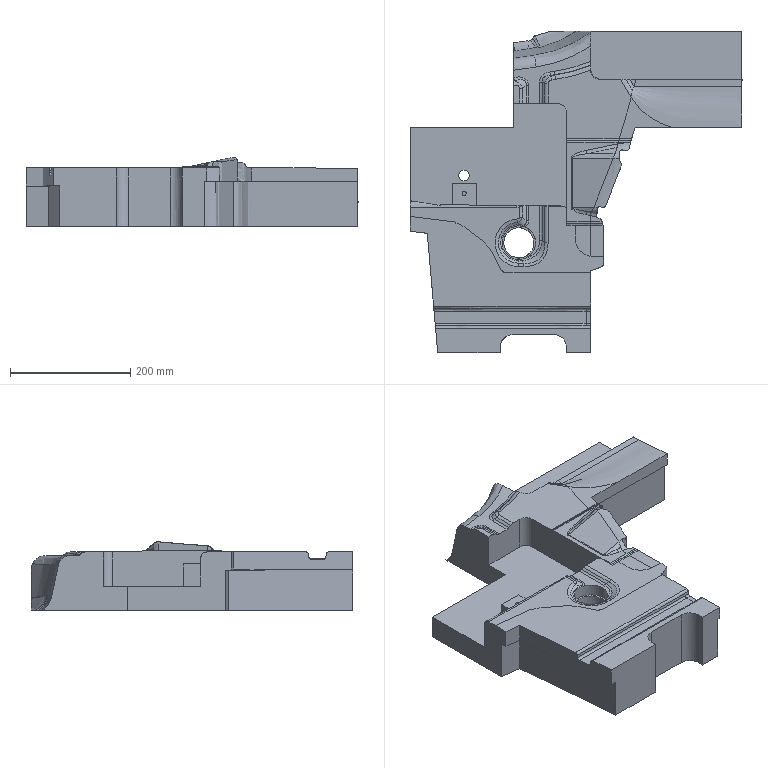Part | NX | features solid 2 | 1 solid | 173 faces | box 552.249 x 535.003 x 114.074 mm | volume 12312889 mm3 | spline 148 | plane 19 | cylinder 6 | commonest cylinder face diameters 40 x2 7 x1 18 x1 30 x1 56 x1